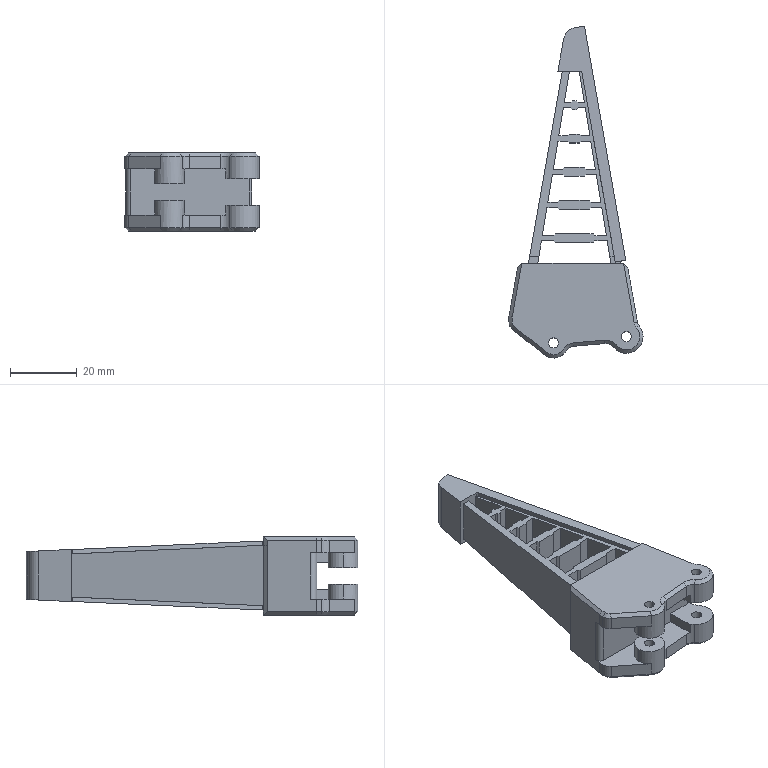Part | SolidWorks | features BaseBody 2, Cut 1 | 2 solids | 208 faces | box 40.322 x 99.83 x 23.5 mm | volume 23198 mm3 | plane 152 | cylinder 43 | cone 13 | commonest cylinder face diameters 3 x9 3.04 x8 2.5 x6 6 x6 9 x4 10 x4